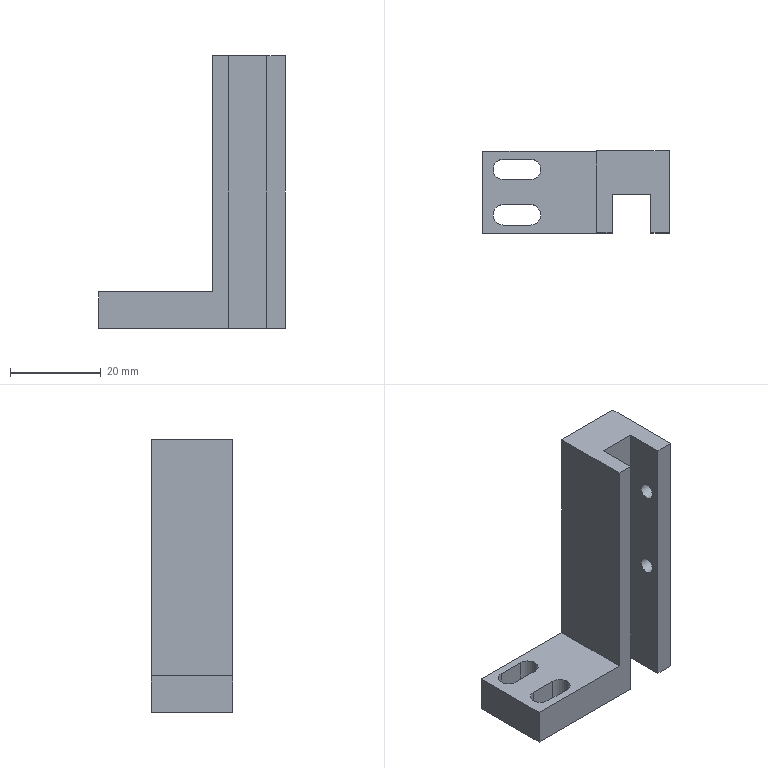Part | NX | features BREP 1 | 1 solid | 22 faces | box 41 x 18 x 60 mm | volume 15782 mm3 | plane 16 | cylinder 6 | commonest cylinder face diameters 4.5 x4 3.5 x2
STEP:
#1=CARTESIAN_POINT('',(-20.5,-9.,-30.));
#2=VERTEX_POINT('',#1);
#3=CARTESIAN_POINT('',(8.,-9.,-30.));
#4=VERTEX_POINT('',#3);
#5=CARTESIAN_POINT('',(-20.5,-9.,-30.));
#6=DIRECTION('',(1.,0.,0.));
#7=VECTOR('',#6,1000.);
#8=LINE('',#5,#7);
#9=EDGE_CURVE('',#2,#4,#8,.T.);
#10=ORIENTED_EDGE('',*,*,#9,.T.);
#11=CARTESIAN_POINT('',(8.,-9.,30.));
#12=VERTEX_POINT('',#11);
#13=CARTESIAN_POINT('',(8.,-9.,-42.021));
#14=DIRECTION('',(0.,0.,1.));
#15=VECTOR('',#14,1000.);
#16=LINE('',#13,#15);
#17=EDGE_CURVE('',#4,#12,#16,.T.);
#18=ORIENTED_EDGE('',*,*,#17,.T.);
#19=CARTESIAN_POINT('',(4.5,-9.,30.));
#20=VERTEX_POINT('',#19);
#21=CARTESIAN_POINT('',(-20.5,-9.,30.));
#22=DIRECTION('',(1.,0.,0.));
#23=VECTOR('',#22,1000.);
#24=LINE('',#21,#23);
#25=EDGE_CURVE('',#20,#12,#24,.T.);
#26=ORIENTED_EDGE('',*,*,#25,.F.);
#27=CARTESIAN_POINT('',(4.5,-9.,-22.));
#28=VERTEX_POINT('',#27);
#29=CARTESIAN_POINT('',(4.5,-9.,30.));
#30=DIRECTION('',(0.,0.,1.));
#31=VECTOR('',#30,1000.);
#32=LINE('',#29,#31);
#33=EDGE_CURVE('',#28,#20,#32,.T.);
#34=ORIENTED_EDGE('',*,*,#33,.F.);
#35=CARTESIAN_POINT('',(-20.5,-9.,-22.));
#36=VERTEX_POINT('',#35);
#37=CARTESIAN_POINT('',(-20.5,-9.,-22.));
#38=DIRECTION('',(1.,0.,0.));
#39=VECTOR('',#38,1000.);
#40=LINE('',#37,#39);
#41=EDGE_CURVE('',#36,#28,#40,.T.);
#42=ORIENTED_EDGE('',*,*,#41,.F.);
#43=CARTESIAN_POINT('',(-20.5,-9.,30.));
#44=DIRECTION('',(0.,0.,-1.));
#45=VECTOR('',#44,1000.);
#46=LINE('',#43,#45);
#47=EDGE_CURVE('',#36,#2,#46,.T.);
#48=ORIENTED_EDGE('',*,*,#47,.T.);
#49=EDGE_LOOP('',(#10,#18,#26,#34,#42,#48));
#50=FACE_BOUND('',#49,.T.);
#51=CARTESIAN_POINT('',(-20.5,-9.,30.));
#52=DIRECTION('',(0.,1.,0.));
#53=DIRECTION('',(0.,0.,-1.));
#54=AXIS2_PLACEMENT_3D('',#51,#52,#53);
#55=PLANE('',#54);
#56=ADVANCED_FACE('',(#50),#55,.F.);
#57=CARTESIAN_POINT('',(20.5,-5.5,-4.45));
#58=VERTEX_POINT('',#57);
#59=CARTESIAN_POINT('',(20.5,-5.5,-2.7));
#60=DIRECTION('',(1.,0.,0.));
#61=DIRECTION('',(0.,0.,-1.));
#62=AXIS2_PLACEMENT_3D('',#59,#60,#61);
#63=CIRCLE('',#62,1.75);
#64=EDGE_CURVE('',#58,#58,#63,.T.);
#65=ORIENTED_EDGE('',*,*,#64,.F.);
#66=EDGE_LOOP('',(#65));
#67=FACE_BOUND('',#66,.T.);
#68=CARTESIAN_POINT('',(20.5,-5.5,15.55));
#69=VERTEX_POINT('',#68);
#70=CARTESIAN_POINT('',(20.5,-5.5,17.3));
#71=DIRECTION('',(1.,0.,0.));
#72=DIRECTION('',(0.,0.,-1.));
#73=AXIS2_PLACEMENT_3D('',#70,#71,#72);
#74=CIRCLE('',#73,1.75);
#75=EDGE_CURVE('',#69,#69,#74,.T.);
#76=ORIENTED_EDGE('',*,*,#75,.F.);
#77=EDGE_LOOP('',(#76));
#78=FACE_BOUND('',#77,.T.);
#79=CARTESIAN_POINT('',(20.5,-9.,-30.));
#80=VERTEX_POINT('',#79);
#81=CARTESIAN_POINT('',(20.5,9.,-30.));
#82=VERTEX_POINT('',#81);
#83=CARTESIAN_POINT('',(20.5,-9.,-30.));
#84=DIRECTION('',(0.,1.,0.));
#85=VECTOR('',#84,1000.);
#86=LINE('',#83,#85);
#87=EDGE_CURVE('',#80,#82,#86,.T.);
#88=ORIENTED_EDGE('',*,*,#87,.T.);
#89=CARTESIAN_POINT('',(20.5,9.,30.));
#90=VERTEX_POINT('',#89);
#91=CARTESIAN_POINT('',(20.5,9.,30.));
#92=DIRECTION('',(0.,0.,-1.));
#93=VECTOR('',#92,1000.);
#94=LINE('',#91,#93);
#95=EDGE_CURVE('',#90,#82,#94,.T.);
#96=ORIENTED_EDGE('',*,*,#95,.F.);
#97=CARTESIAN_POINT('',(20.5,-9.,30.));
#98=VERTEX_POINT('',#97);
#99=CARTESIAN_POINT('',(20.5,-9.,30.));
#100=DIRECTION('',(0.,1.,0.));
#101=VECTOR('',#100,1000.);
#102=LINE('',#99,#101);
#103=EDGE_CURVE('',#98,#90,#102,.T.);
#104=ORIENTED_EDGE('',*,*,#103,.F.);
#105=CARTESIAN_POINT('',(20.5,-9.,30.));
#106=DIRECTION('',(0.,0.,-1.));
#107=VECTOR('',#106,1000.);
#108=LINE('',#105,#107);
#109=EDGE_CURVE('',#98,#80,#108,.T.);
#110=ORIENTED_EDGE('',*,*,#109,.T.);
#111=EDGE_LOOP('',(#88,#96,#104,#110));
#112=FACE_BOUND('',#111,.T.);
#113=CARTESIAN_POINT('',(20.5,-9.,30.));
#114=DIRECTION('',(-1.,0.,0.));
#115=DIRECTION('',(0.,0.,-1.));
#116=AXIS2_PLACEMENT_3D('',#113,#114,#115);
#117=PLANE('',#116);
#118=ADVANCED_FACE('',(#67,#78,#112),#117,.F.);
#119=CARTESIAN_POINT('',(-20.5,9.,-22.));
#120=VERTEX_POINT('',#119);
#121=CARTESIAN_POINT('',(-20.5,9.,-30.));
#122=VERTEX_POINT('',#121);
#123=CARTESIAN_POINT('',(-20.5,9.,30.));
#124=DIRECTION('',(0.,0.,-1.));
#125=VECTOR('',#124,1000.);
#126=LINE('',#123,#125);
#127=EDGE_CURVE('',#120,#122,#126,.T.);
#128=ORIENTED_EDGE('',*,*,#127,.F.);
#129=CARTESIAN_POINT('',(4.5,9.,-22.));
#130=VERTEX_POINT('',#129);
#131=CARTESIAN_POINT('',(-20.5,9.,-22.));
#132=DIRECTION('',(-1.,0.,0.));
#133=VECTOR('',#132,1000.);
#134=LINE('',#131,#133);
#135=EDGE_CURVE('',#130,#120,#134,.T.);
#136=ORIENTED_EDGE('',*,*,#135,.F.);
#137=CARTESIAN_POINT('',(4.5,9.,30.));
#138=VERTEX_POINT('',#137);
#139=CARTESIAN_POINT('',(4.5,9.,30.));
#140=DIRECTION('',(0.,0.,-1.));
#141=VECTOR('',#140,1000.);
#142=LINE('',#139,#141);
#143=EDGE_CURVE('',#138,#130,#142,.T.);
#144=ORIENTED_EDGE('',*,*,#143,.F.);
#145=CARTESIAN_POINT('',(-20.5,9.,30.));
#146=DIRECTION('',(-1.,0.,0.));
#147=VECTOR('',#146,1000.);
#148=LINE('',#145,#147);
#149=EDGE_CURVE('',#90,#138,#148,.T.);
#150=ORIENTED_EDGE('',*,*,#149,.F.);
#151=ORIENTED_EDGE('',*,*,#95,.T.);
#152=CARTESIAN_POINT('',(-20.5,9.,-30.));
#153=DIRECTION('',(-1.,0.,0.));
#154=VECTOR('',#153,1000.);
#155=LINE('',#152,#154);
#156=EDGE_CURVE('',#82,#122,#155,.T.);
#157=ORIENTED_EDGE('',*,*,#156,.T.);
#158=EDGE_LOOP('',(#128,#136,#144,#150,#151,#157));
#159=FACE_BOUND('',#158,.T.);
#160=CARTESIAN_POINT('',(-20.5,9.,30.));
#161=DIRECTION('',(0.,-1.,0.));
#162=DIRECTION('',(0.,0.,1.));
#163=AXIS2_PLACEMENT_3D('',#160,#161,#162);
#164=PLANE('',#163);
#165=ADVANCED_FACE('',(#159),#164,.F.);
#166=ORIENTED_EDGE('',*,*,#47,.F.);
#167=CARTESIAN_POINT('',(-20.5,-66.697,-22.));
#168=DIRECTION('',(0.,1.,0.));
#169=VECTOR('',#168,1000.);
#170=LINE('',#167,#169);
#171=EDGE_CURVE('',#36,#120,#170,.T.);
#172=ORIENTED_EDGE('',*,*,#171,.T.);
#173=ORIENTED_EDGE('',*,*,#127,.T.);
#174=CARTESIAN_POINT('',(-20.5,-9.,-30.));
#175=DIRECTION('',(0.,-1.,0.));
#176=VECTOR('',#175,1000.);
#177=LINE('',#174,#176);
#178=EDGE_CURVE('',#122,#2,#177,.T.);
#179=ORIENTED_EDGE('',*,*,#178,.T.);
#180=EDGE_LOOP('',(#166,#172,#173,#179));
#181=FACE_BOUND('',#180,.T.);
#182=CARTESIAN_POINT('',(-20.5,-9.,30.));
#183=DIRECTION('',(1.,0.,0.));
#184=DIRECTION('',(0.,0.,1.));
#185=AXIS2_PLACEMENT_3D('',#182,#183,#184);
#186=PLANE('',#185);
#187=ADVANCED_FACE('',(#181),#186,.F.);
#188=CARTESIAN_POINT('',(16.5,-9.,30.));
#189=VERTEX_POINT('',#188);
#190=CARTESIAN_POINT('',(-20.5,-9.,30.));
#191=DIRECTION('',(1.,0.,0.));
#192=VECTOR('',#191,1000.);
#193=LINE('',#190,#192);
#194=EDGE_CURVE('',#189,#98,#193,.T.);
#195=ORIENTED_EDGE('',*,*,#194,.F.);
#196=CARTESIAN_POINT('',(16.5,-9.,-30.));
#197=VERTEX_POINT('',#196);
#198=CARTESIAN_POINT('',(16.5,-9.,-42.021));
#199=DIRECTION('',(0.,0.,1.));
#200=VECTOR('',#199,1000.);
#201=LINE('',#198,#200);
#202=EDGE_CURVE('',#197,#189,#201,.T.);
#203=ORIENTED_EDGE('',*,*,#202,.F.);
#204=CARTESIAN_POINT('',(-20.5,-9.,-30.));
#205=DIRECTION('',(1.,0.,0.));
#206=VECTOR('',#205,1000.);
#207=LINE('',#204,#206);
#208=EDGE_CURVE('',#197,#80,#207,.T.);
#209=ORIENTED_EDGE('',*,*,#208,.T.);
#210=ORIENTED_EDGE('',*,*,#109,.F.);
#211=EDGE_LOOP('',(#195,#203,#209,#210));
#212=FACE_BOUND('',#211,.T.);
#213=CARTESIAN_POINT('',(-20.5,-9.,30.));
#214=DIRECTION('',(0.,1.,0.));
#215=DIRECTION('',(0.,0.,-1.));
#216=AXIS2_PLACEMENT_3D('',#213,#214,#215);
#217=PLANE('',#216);
#218=ADVANCED_FACE('',(#212),#217,.F.);
#219=ORIENTED_EDGE('',*,*,#25,.T.);
#220=CARTESIAN_POINT('',(8.,-0.5,30.));
#221=VERTEX_POINT('',#220);
#222=CARTESIAN_POINT('',(8.,-9.,30.));
#223=DIRECTION('',(0.,-1.,0.));
#224=VECTOR('',#223,1000.);
#225=LINE('',#222,#224);
#226=EDGE_CURVE('',#221,#12,#225,.T.);
#227=ORIENTED_EDGE('',*,*,#226,.F.);
#228=CARTESIAN_POINT('',(16.5,-0.5,30.));
#229=VERTEX_POINT('',#228);
#230=CARTESIAN_POINT('',(16.5,-0.5,30.));
#231=DIRECTION('',(-1.,0.,0.));
#232=VECTOR('',#231,1000.);
#233=LINE('',#230,#232);
#234=EDGE_CURVE('',#229,#221,#233,.T.);
#235=ORIENTED_EDGE('',*,*,#234,.F.);
#236=CARTESIAN_POINT('',(16.5,-9.,30.));
#237=DIRECTION('',(0.,1.,0.));
#238=VECTOR('',#237,1000.);
#239=LINE('',#236,#238);
#240=EDGE_CURVE('',#189,#229,#239,.T.);
#241=ORIENTED_EDGE('',*,*,#240,.F.);
#242=ORIENTED_EDGE('',*,*,#194,.T.);
#243=ORIENTED_EDGE('',*,*,#103,.T.);
#244=ORIENTED_EDGE('',*,*,#149,.T.);
#245=CARTESIAN_POINT('',(4.5,-66.697,30.));
#246=DIRECTION('',(0.,1.,0.));
#247=VECTOR('',#246,1000.);
#248=LINE('',#245,#247);
#249=EDGE_CURVE('',#20,#138,#248,.T.);
#250=ORIENTED_EDGE('',*,*,#249,.F.);
#251=EDGE_LOOP('',(#219,#227,#235,#241,#242,#243,#244,#250));
#252=FACE_BOUND('',#251,.T.);
#253=CARTESIAN_POINT('',(0.,0.,30.));
#254=DIRECTION('',(0.,0.,-1.));
#255=DIRECTION('',(1.,0.,0.));
#256=AXIS2_PLACEMENT_3D('',#253,#254,#255);
#257=PLANE('',#256);
#258=ADVANCED_FACE('',(#252),#257,.F.);
#259=CARTESIAN_POINT('',(-16.,-7.25,-30.));
#260=VERTEX_POINT('',#259);
#261=CARTESIAN_POINT('',(-16.,-2.75,-30.));
#262=VERTEX_POINT('',#261);
#263=CARTESIAN_POINT('',(-16.,-5.,-30.));
#264=DIRECTION('',(0.,0.,-1.));
#265=DIRECTION('',(-1.,0.,0.));
#266=AXIS2_PLACEMENT_3D('',#263,#264,#265);
#267=CIRCLE('',#266,2.25);
#268=EDGE_CURVE('',#260,#262,#267,.T.);
#269=ORIENTED_EDGE('',*,*,#268,.F.);
#270=CARTESIAN_POINT('',(-10.,-7.25,-30.));
#271=VERTEX_POINT('',#270);
#272=CARTESIAN_POINT('',(-16.,-7.25,-30.));
#273=DIRECTION('',(-1.,0.,0.));
#274=VECTOR('',#273,1000.);
#275=LINE('',#272,#274);
#276=EDGE_CURVE('',#271,#260,#275,.T.);
#277=ORIENTED_EDGE('',*,*,#276,.F.);
#278=CARTESIAN_POINT('',(-10.,-2.75,-30.));
#279=VERTEX_POINT('',#278);
#280=CARTESIAN_POINT('',(-10.,-5.,-30.));
#281=DIRECTION('',(0.,0.,-1.));
#282=DIRECTION('',(-1.,0.,0.));
#283=AXIS2_PLACEMENT_3D('',#280,#281,#282);
#284=CIRCLE('',#283,2.25);
#285=EDGE_CURVE('',#279,#271,#284,.T.);
#286=ORIENTED_EDGE('',*,*,#285,.F.);
#287=CARTESIAN_POINT('',(-16.,-2.75,-30.));
#288=DIRECTION('',(1.,0.,0.));
#289=VECTOR('',#288,1000.);
#290=LINE('',#287,#289);
#291=EDGE_CURVE('',#262,#279,#290,.T.);
#292=ORIENTED_EDGE('',*,*,#291,.F.);
#293=EDGE_LOOP('',(#269,#277,#286,#292));
#294=FACE_BOUND('',#293,.T.);
#295=CARTESIAN_POINT('',(-16.,2.75,-30.));
#296=VERTEX_POINT('',#295);
#297=CARTESIAN_POINT('',(-16.,7.25,-30.));
#298=VERTEX_POINT('',#297);
#299=CARTESIAN_POINT('',(-16.,5.,-30.));
#300=DIRECTION('',(0.,0.,-1.));
#301=DIRECTION('',(-1.,0.,0.));
#302=AXIS2_PLACEMENT_3D('',#299,#300,#301);
#303=CIRCLE('',#302,2.25);
#304=EDGE_CURVE('',#296,#298,#303,.T.);
#305=ORIENTED_EDGE('',*,*,#304,.F.);
#306=CARTESIAN_POINT('',(-10.,2.75,-30.));
#307=VERTEX_POINT('',#306);
#308=CARTESIAN_POINT('',(-16.,2.75,-30.));
#309=DIRECTION('',(-1.,0.,0.));
#310=VECTOR('',#309,1000.);
#311=LINE('',#308,#310);
#312=EDGE_CURVE('',#307,#296,#311,.T.);
#313=ORIENTED_EDGE('',*,*,#312,.F.);
#314=CARTESIAN_POINT('',(-10.,7.25,-30.));
#315=VERTEX_POINT('',#314);
#316=CARTESIAN_POINT('',(-10.,5.,-30.));
#317=DIRECTION('',(0.,0.,-1.));
#318=DIRECTION('',(-1.,0.,0.));
#319=AXIS2_PLACEMENT_3D('',#316,#317,#318);
#320=CIRCLE('',#319,2.25);
#321=EDGE_CURVE('',#315,#307,#320,.T.);
#322=ORIENTED_EDGE('',*,*,#321,.F.);
#323=CARTESIAN_POINT('',(-16.,7.25,-30.));
#324=DIRECTION('',(1.,0.,0.));
#325=VECTOR('',#324,1000.);
#326=LINE('',#323,#325);
#327=EDGE_CURVE('',#298,#315,#326,.T.);
#328=ORIENTED_EDGE('',*,*,#327,.F.);
#329=EDGE_LOOP('',(#305,#313,#322,#328));
#330=FACE_BOUND('',#329,.T.);
#331=CARTESIAN_POINT('',(8.,-0.5,-30.));
#332=VERTEX_POINT('',#331);
#333=CARTESIAN_POINT('',(8.,-9.,-30.));
#334=DIRECTION('',(0.,-1.,0.));
#335=VECTOR('',#334,1000.);
#336=LINE('',#333,#335);
#337=EDGE_CURVE('',#332,#4,#336,.T.);
#338=ORIENTED_EDGE('',*,*,#337,.T.);
#339=ORIENTED_EDGE('',*,*,#9,.F.);
#340=ORIENTED_EDGE('',*,*,#178,.F.);
#341=ORIENTED_EDGE('',*,*,#156,.F.);
#342=ORIENTED_EDGE('',*,*,#87,.F.);
#343=ORIENTED_EDGE('',*,*,#208,.F.);
#344=CARTESIAN_POINT('',(16.5,-0.5,-30.));
#345=VERTEX_POINT('',#344);
#346=CARTESIAN_POINT('',(16.5,-9.,-30.));
#347=DIRECTION('',(0.,1.,0.));
#348=VECTOR('',#347,1000.);
#349=LINE('',#346,#348);
#350=EDGE_CURVE('',#197,#345,#349,.T.);
#351=ORIENTED_EDGE('',*,*,#350,.T.);
#352=CARTESIAN_POINT('',(16.5,-0.5,-30.));
#353=DIRECTION('',(-1.,0.,0.));
#354=VECTOR('',#353,1000.);
#355=LINE('',#352,#354);
#356=EDGE_CURVE('',#345,#332,#355,.T.);
#357=ORIENTED_EDGE('',*,*,#356,.T.);
#358=EDGE_LOOP('',(#338,#339,#340,#341,#342,#343,#351,#357));
#359=FACE_BOUND('',#358,.T.);
#360=CARTESIAN_POINT('',(0.,0.,-30.));
#361=DIRECTION('',(0.,0.,-1.));
#362=DIRECTION('',(1.,0.,0.));
#363=AXIS2_PLACEMENT_3D('',#360,#361,#362);
#364=PLANE('',#363);
#365=ADVANCED_FACE('',(#294,#330,#359),#364,.T.);
#366=CARTESIAN_POINT('',(-16.,-7.25,-22.));
#367=VERTEX_POINT('',#366);
#368=CARTESIAN_POINT('',(-10.,-7.25,-22.));
#369=VERTEX_POINT('',#368);
#370=CARTESIAN_POINT('',(-16.,-7.25,-22.));
#371=DIRECTION('',(1.,0.,0.));
#372=VECTOR('',#371,1000.);
#373=LINE('',#370,#372);
#374=EDGE_CURVE('',#367,#369,#373,.T.);
#375=ORIENTED_EDGE('',*,*,#374,.F.);
#376=CARTESIAN_POINT('',(-16.,-2.75,-22.));
#377=VERTEX_POINT('',#376);
#378=CARTESIAN_POINT('',(-16.,-5.,-22.));
#379=DIRECTION('',(0.,0.,1.));
#380=DIRECTION('',(-1.,0.,0.));
#381=AXIS2_PLACEMENT_3D('',#378,#379,#380);
#382=CIRCLE('',#381,2.25);
#383=EDGE_CURVE('',#377,#367,#382,.T.);
#384=ORIENTED_EDGE('',*,*,#383,.F.);
#385=CARTESIAN_POINT('',(-10.,-2.75,-22.));
#386=VERTEX_POINT('',#385);
#387=CARTESIAN_POINT('',(-16.,-2.75,-22.));
#388=DIRECTION('',(-1.,0.,0.));
#389=VECTOR('',#388,1000.);
#390=LINE('',#387,#389);
#391=EDGE_CURVE('',#386,#377,#390,.T.);
#392=ORIENTED_EDGE('',*,*,#391,.F.);
#393=CARTESIAN_POINT('',(-10.,-5.,-22.));
#394=DIRECTION('',(0.,0.,1.));
#395=DIRECTION('',(-1.,0.,0.));
#396=AXIS2_PLACEMENT_3D('',#393,#394,#395);
#397=CIRCLE('',#396,2.25);
#398=EDGE_CURVE('',#369,#386,#397,.T.);
#399=ORIENTED_EDGE('',*,*,#398,.F.);
#400=EDGE_LOOP('',(#375,#384,#392,#399));
#401=FACE_BOUND('',#400,.T.);
#402=CARTESIAN_POINT('',(-16.,2.75,-22.));
#403=VERTEX_POINT('',#402);
#404=CARTESIAN_POINT('',(-10.,2.75,-22.));
#405=VERTEX_POINT('',#404);
#406=CARTESIAN_POINT('',(-16.,2.75,-22.));
#407=DIRECTION('',(1.,0.,0.));
#408=VECTOR('',#407,1000.);
#409=LINE('',#406,#408);
#410=EDGE_CURVE('',#403,#405,#409,.T.);
#411=ORIENTED_EDGE('',*,*,#410,.F.);
#412=CARTESIAN_POINT('',(-16.,7.25,-22.));
#413=VERTEX_POINT('',#412);
#414=CARTESIAN_POINT('',(-16.,5.,-22.));
#415=DIRECTION('',(0.,0.,1.));
#416=DIRECTION('',(-1.,0.,0.));
#417=AXIS2_PLACEMENT_3D('',#414,#415,#416);
#418=CIRCLE('',#417,2.25);
#419=EDGE_CURVE('',#413,#403,#418,.T.);
#420=ORIENTED_EDGE('',*,*,#419,.F.);
#421=CARTESIAN_POINT('',(-10.,7.25,-22.));
#422=VERTEX_POINT('',#421);
#423=CARTESIAN_POINT('',(-16.,7.25,-22.));
#424=DIRECTION('',(-1.,0.,0.));
#425=VECTOR('',#424,1000.);
#426=LINE('',#423,#425);
#427=EDGE_CURVE('',#422,#413,#426,.T.);
#428=ORIENTED_EDGE('',*,*,#427,.F.);
#429=CARTESIAN_POINT('',(-10.,5.,-22.));
#430=DIRECTION('',(0.,0.,1.));
#431=DIRECTION('',(-1.,0.,0.));
#432=AXIS2_PLACEMENT_3D('',#429,#430,#431);
#433=CIRCLE('',#432,2.25);
#434=EDGE_CURVE('',#405,#422,#433,.T.);
#435=ORIENTED_EDGE('',*,*,#434,.F.);
#436=EDGE_LOOP('',(#411,#420,#428,#435));
#437=FACE_BOUND('',#436,.T.);
#438=ORIENTED_EDGE('',*,*,#41,.T.);
#439=CARTESIAN_POINT('',(4.5,-66.697,-22.));
#440=DIRECTION('',(0.,1.,0.));
#441=VECTOR('',#440,1000.);
#442=LINE('',#439,#441);
#443=EDGE_CURVE('',#28,#130,#442,.T.);
#444=ORIENTED_EDGE('',*,*,#443,.T.);
#445=ORIENTED_EDGE('',*,*,#135,.T.);
#446=ORIENTED_EDGE('',*,*,#171,.F.);
#447=EDGE_LOOP('',(#438,#444,#445,#446));
#448=FACE_BOUND('',#447,.T.);
#449=CARTESIAN_POINT('',(-20.5,-66.697,-22.));
#450=DIRECTION('',(0.,0.,-1.));
#451=DIRECTION('',(1.,0.,0.));
#452=AXIS2_PLACEMENT_3D('',#449,#450,#451);
#453=PLANE('',#452);
#454=ADVANCED_FACE('',(#401,#437,#448),#453,.F.);
#455=ORIENTED_EDGE('',*,*,#33,.T.);
#456=ORIENTED_EDGE('',*,*,#249,.T.);
#457=ORIENTED_EDGE('',*,*,#143,.T.);
#458=ORIENTED_EDGE('',*,*,#443,.F.);
#459=EDGE_LOOP('',(#455,#456,#457,#458));
#460=FACE_BOUND('',#459,.T.);
#461=CARTESIAN_POINT('',(4.5,-66.697,30.));
#462=DIRECTION('',(1.,0.,0.));
#463=DIRECTION('',(0.,0.,1.));
#464=AXIS2_PLACEMENT_3D('',#461,#462,#463);
#465=PLANE('',#464);
#466=ADVANCED_FACE('',(#460),#465,.F.);
#467=CARTESIAN_POINT('',(16.5,-0.5,-42.021));
#468=DIRECTION('',(0.,0.,1.));
#469=VECTOR('',#468,1000.);
#470=LINE('',#467,#469);
#471=EDGE_CURVE('',#345,#229,#470,.T.);
#472=ORIENTED_EDGE('',*,*,#471,.T.);
#473=ORIENTED_EDGE('',*,*,#234,.T.);
#474=CARTESIAN_POINT('',(8.,-0.5,-42.021));
#475=DIRECTION('',(0.,0.,1.));
#476=VECTOR('',#475,1000.);
#477=LINE('',#474,#476);
#478=EDGE_CURVE('',#332,#221,#477,.T.);
#479=ORIENTED_EDGE('',*,*,#478,.F.);
#480=ORIENTED_EDGE('',*,*,#356,.F.);
#481=EDGE_LOOP('',(#472,#473,#479,#480));
#482=FACE_BOUND('',#481,.T.);
#483=CARTESIAN_POINT('',(16.5,-0.5,-42.021));
#484=DIRECTION('',(0.,1.,0.));
#485=DIRECTION('',(1.,0.,0.));
#486=AXIS2_PLACEMENT_3D('',#483,#484,#485);
#487=PLANE('',#486);
#488=ADVANCED_FACE('',(#482),#487,.F.);
#489=ORIENTED_EDGE('',*,*,#478,.T.);
#490=ORIENTED_EDGE('',*,*,#226,.T.);
#491=ORIENTED_EDGE('',*,*,#17,.F.);
#492=ORIENTED_EDGE('',*,*,#337,.F.);
#493=EDGE_LOOP('',(#489,#490,#491,#492));
#494=FACE_BOUND('',#493,.T.);
#495=CARTESIAN_POINT('',(8.,-9.,-42.021));
#496=DIRECTION('',(-1.,0.,0.));
#497=DIRECTION('',(0.,0.,-1.));
#498=AXIS2_PLACEMENT_3D('',#495,#496,#497);
#499=PLANE('',#498);
#500=ADVANCED_FACE('',(#494),#499,.F.);
#501=CARTESIAN_POINT('',(16.5,-5.5,-4.45));
#502=VERTEX_POINT('',#501);
#503=CARTESIAN_POINT('',(16.5,-5.5,-2.7));
#504=DIRECTION('',(1.,0.,0.));
#505=DIRECTION('',(0.,0.,-1.));
#506=AXIS2_PLACEMENT_3D('',#503,#504,#505);
#507=CIRCLE('',#506,1.75);
#508=EDGE_CURVE('',#502,#502,#507,.T.);
#509=ORIENTED_EDGE('',*,*,#508,.T.);
#510=EDGE_LOOP('',(#509));
#511=FACE_BOUND('',#510,.T.);
#512=CARTESIAN_POINT('',(16.5,-5.5,15.55));
#513=VERTEX_POINT('',#512);
#514=CARTESIAN_POINT('',(16.5,-5.5,17.3));
#515=DIRECTION('',(1.,0.,0.));
#516=DIRECTION('',(0.,0.,-1.));
#517=AXIS2_PLACEMENT_3D('',#514,#515,#516);
#518=CIRCLE('',#517,1.75);
#519=EDGE_CURVE('',#513,#513,#518,.T.);
#520=ORIENTED_EDGE('',*,*,#519,.T.);
#521=EDGE_LOOP('',(#520));
#522=FACE_BOUND('',#521,.T.);
#523=ORIENTED_EDGE('',*,*,#202,.T.);
#524=ORIENTED_EDGE('',*,*,#240,.T.);
#525=ORIENTED_EDGE('',*,*,#471,.F.);
#526=ORIENTED_EDGE('',*,*,#350,.F.);
#527=EDGE_LOOP('',(#523,#524,#525,#526));
#528=FACE_BOUND('',#527,.T.);
#529=CARTESIAN_POINT('',(16.5,-9.,-42.021));
#530=DIRECTION('',(1.,0.,0.));
#531=DIRECTION('',(0.,0.,1.));
#532=AXIS2_PLACEMENT_3D('',#529,#530,#531);
#533=PLANE('',#532);
#534=ADVANCED_FACE('',(#511,#522,#528),#533,.F.);
#535=ORIENTED_EDGE('',*,*,#419,.T.);
#536=CARTESIAN_POINT('',(-16.,2.75,-10.576));
#537=DIRECTION('',(0.,0.,-1.));
#538=VECTOR('',#537,1000.);
#539=LINE('',#536,#538);
#540=EDGE_CURVE('',#403,#296,#539,.T.);
#541=ORIENTED_EDGE('',*,*,#540,.T.);
#542=ORIENTED_EDGE('',*,*,#304,.T.);
#543=CARTESIAN_POINT('',(-16.,7.25,-10.576));
#544=DIRECTION('',(0.,0.,-1.));
#545=VECTOR('',#544,1000.);
#546=LINE('',#543,#545);
#547=EDGE_CURVE('',#413,#298,#546,.T.);
#548=ORIENTED_EDGE('',*,*,#547,.F.);
#549=EDGE_LOOP('',(#535,#541,#542,#548));
#550=FACE_BOUND('',#549,.T.);
#551=CARTESIAN_POINT('',(-16.,5.,-10.576));
#552=DIRECTION('',(0.,0.,-1.));
#553=DIRECTION('',(1.,0.,0.));
#554=AXIS2_PLACEMENT_3D('',#551,#552,#553);
#555=CYLINDRICAL_SURFACE('',#554,2.25);
#556=ADVANCED_FACE('',(#550),#555,.F.);
#557=ORIENTED_EDGE('',*,*,#410,.T.);
#558=CARTESIAN_POINT('',(-10.,2.75,-10.576));
#559=DIRECTION('',(0.,0.,-1.));
#560=VECTOR('',#559,1000.);
#561=LINE('',#558,#560);
#562=EDGE_CURVE('',#405,#307,#561,.T.);
#563=ORIENTED_EDGE('',*,*,#562,.T.);
#564=ORIENTED_EDGE('',*,*,#312,.T.);
#565=ORIENTED_EDGE('',*,*,#540,.F.);
#566=EDGE_LOOP('',(#557,#563,#564,#565));
#567=FACE_BOUND('',#566,.T.);
#568=CARTESIAN_POINT('',(-16.,2.75,-10.576));
#569=DIRECTION('',(0.,-1.,0.));
#570=DIRECTION('',(-1.,0.,0.));
#571=AXIS2_PLACEMENT_3D('',#568,#569,#570);
#572=PLANE('',#571);
#573=ADVANCED_FACE('',(#567),#572,.F.);
#574=ORIENTED_EDGE('',*,*,#434,.T.);
#575=CARTESIAN_POINT('',(-10.,7.25,-10.576));
#576=DIRECTION('',(0.,0.,-1.));
#577=VECTOR('',#576,1000.);
#578=LINE('',#575,#577);
#579=EDGE_CURVE('',#422,#315,#578,.T.);
#580=ORIENTED_EDGE('',*,*,#579,.T.);
#581=ORIENTED_EDGE('',*,*,#321,.T.);
#582=ORIENTED_EDGE('',*,*,#562,.F.);
#583=EDGE_LOOP('',(#574,#580,#581,#582));
#584=FACE_BOUND('',#583,.T.);
#585=CARTESIAN_POINT('',(-10.,5.,-10.576));
#586=DIRECTION('',(0.,0.,-1.));
#587=DIRECTION('',(1.,0.,0.));
#588=AXIS2_PLACEMENT_3D('',#585,#586,#587);
#589=CYLINDRICAL_SURFACE('',#588,2.25);
#590=ADVANCED_FACE('',(#584),#589,.F.);
#591=ORIENTED_EDGE('',*,*,#427,.T.);
#592=ORIENTED_EDGE('',*,*,#547,.T.);
#593=ORIENTED_EDGE('',*,*,#327,.T.);
#594=ORIENTED_EDGE('',*,*,#579,.F.);
#595=EDGE_LOOP('',(#591,#592,#593,#594));
#596=FACE_BOUND('',#595,.T.);
#597=CARTESIAN_POINT('',(-16.,7.25,-10.576));
#598=DIRECTION('',(0.,1.,0.));
#599=DIRECTION('',(1.,0.,0.));
#600=AXIS2_PLACEMENT_3D('',#597,#598,#599);
#601=PLANE('',#600);
#602=ADVANCED_FACE('',(#596),#601,.F.);
#603=ORIENTED_EDGE('',*,*,#383,.T.);
#604=CARTESIAN_POINT('',(-16.,-7.25,-10.576));
#605=DIRECTION('',(0.,0.,-1.));
#606=VECTOR('',#605,1000.);
#607=LINE('',#604,#606);
#608=EDGE_CURVE('',#367,#260,#607,.T.);
#609=ORIENTED_EDGE('',*,*,#608,.T.);
#610=ORIENTED_EDGE('',*,*,#268,.T.);
#611=CARTESIAN_POINT('',(-16.,-2.75,-10.576));
#612=DIRECTION('',(0.,0.,-1.));
#613=VECTOR('',#612,1000.);
#614=LINE('',#611,#613);
#615=EDGE_CURVE('',#377,#262,#614,.T.);
#616=ORIENTED_EDGE('',*,*,#615,.F.);
#617=EDGE_LOOP('',(#603,#609,#610,#616));
#618=FACE_BOUND('',#617,.T.);
#619=CARTESIAN_POINT('',(-16.,-5.,-10.576));
#620=DIRECTION('',(0.,0.,-1.));
#621=DIRECTION('',(1.,0.,0.));
#622=AXIS2_PLACEMENT_3D('',#619,#620,#621);
#623=CYLINDRICAL_SURFACE('',#622,2.25);
#624=ADVANCED_FACE('',(#618),#623,.F.);
#625=ORIENTED_EDGE('',*,*,#374,.T.);
#626=CARTESIAN_POINT('',(-10.,-7.25,-10.576));
#627=DIRECTION('',(0.,0.,-1.));
#628=VECTOR('',#627,1000.);
#629=LINE('',#626,#628);
#630=EDGE_CURVE('',#369,#271,#629,.T.);
#631=ORIENTED_EDGE('',*,*,#630,.T.);
#632=ORIENTED_EDGE('',*,*,#276,.T.);
#633=ORIENTED_EDGE('',*,*,#608,.F.);
#634=EDGE_LOOP('',(#625,#631,#632,#633));
#635=FACE_BOUND('',#634,.T.);
#636=CARTESIAN_POINT('',(-16.,-7.25,-10.576));
#637=DIRECTION('',(0.,-1.,0.));
#638=DIRECTION('',(-1.,0.,0.));
#639=AXIS2_PLACEMENT_3D('',#636,#637,#638);
#640=PLANE('',#639);
#641=ADVANCED_FACE('',(#635),#640,.F.);
#642=ORIENTED_EDGE('',*,*,#398,.T.);
#643=CARTESIAN_POINT('',(-10.,-2.75,-10.576));
#644=DIRECTION('',(0.,0.,-1.));
#645=VECTOR('',#644,1000.);
#646=LINE('',#643,#645);
#647=EDGE_CURVE('',#386,#279,#646,.T.);
#648=ORIENTED_EDGE('',*,*,#647,.T.);
#649=ORIENTED_EDGE('',*,*,#285,.T.);
#650=ORIENTED_EDGE('',*,*,#630,.F.);
#651=EDGE_LOOP('',(#642,#648,#649,#650));
#652=FACE_BOUND('',#651,.T.);
#653=CARTESIAN_POINT('',(-10.,-5.,-10.576));
#654=DIRECTION('',(0.,0.,-1.));
#655=DIRECTION('',(1.,0.,0.));
#656=AXIS2_PLACEMENT_3D('',#653,#654,#655);
#657=CYLINDRICAL_SURFACE('',#656,2.25);
#658=ADVANCED_FACE('',(#652),#657,.F.);
#659=ORIENTED_EDGE('',*,*,#391,.T.);
#660=ORIENTED_EDGE('',*,*,#615,.T.);
#661=ORIENTED_EDGE('',*,*,#291,.T.);
#662=ORIENTED_EDGE('',*,*,#647,.F.);
#663=EDGE_LOOP('',(#659,#660,#661,#662));
#664=FACE_BOUND('',#663,.T.);
#665=CARTESIAN_POINT('',(-16.,-2.75,-10.576));
#666=DIRECTION('',(0.,1.,0.));
#667=DIRECTION('',(1.,0.,0.));
#668=AXIS2_PLACEMENT_3D('',#665,#666,#667);
#669=PLANE('',#668);
#670=ADVANCED_FACE('',(#664),#669,.F.);
#671=ORIENTED_EDGE('',*,*,#75,.T.);
#672=EDGE_LOOP('',(#671));
#673=FACE_BOUND('',#672,.T.);
#674=ORIENTED_EDGE('',*,*,#519,.F.);
#675=EDGE_LOOP('',(#674));
#676=FACE_BOUND('',#675,.T.);
#677=CARTESIAN_POINT('',(20.5,-5.5,17.3));
#678=DIRECTION('',(1.,0.,0.));
#679=DIRECTION('',(0.,0.,1.));
#680=AXIS2_PLACEMENT_3D('',#677,#678,#679);
#681=CYLINDRICAL_SURFACE('',#680,1.75);
#682=ADVANCED_FACE('',(#673,#676),#681,.F.);
#683=ORIENTED_EDGE('',*,*,#64,.T.);
#684=EDGE_LOOP('',(#683));
#685=FACE_BOUND('',#684,.T.);
#686=ORIENTED_EDGE('',*,*,#508,.F.);
#687=EDGE_LOOP('',(#686));
#688=FACE_BOUND('',#687,.T.);
#689=CARTESIAN_POINT('',(20.5,-5.5,-2.7));
#690=DIRECTION('',(1.,0.,0.));
#691=DIRECTION('',(0.,0.,1.));
#692=AXIS2_PLACEMENT_3D('',#689,#690,#691);
#693=CYLINDRICAL_SURFACE('',#692,1.75);
#694=ADVANCED_FACE('',(#685,#688),#693,.F.);
#695=CLOSED_SHELL('',(#56,#118,#165,#187,#218,#258,#365,#454,#466,#488,#500,#534,#556,#573,#590,#602,#624,#641,#658,#670,#682,#694));
#696=MANIFOLD_SOLID_BREP('',#695);
#697=(LENGTH_UNIT()NAMED_UNIT(*)SI_UNIT(.MILLI.,.METRE.));
#698=UNCERTAINTY_MEASURE_WITH_UNIT(LENGTH_MEASURE(0.00001),#697,'','');
#699=(NAMED_UNIT(*)PLANE_ANGLE_UNIT()SI_UNIT($,.RADIAN.));
#700=(NAMED_UNIT(*)SI_UNIT($,.STERADIAN.)SOLID_ANGLE_UNIT());
#701=(GEOMETRIC_REPRESENTATION_CONTEXT(3)GLOBAL_UNCERTAINTY_ASSIGNED_CONTEXT((#698))GLOBAL_UNIT_ASSIGNED_CONTEXT((#697,#699,#700))REPRESENTATION_CONTEXT('',''));
#702=ADVANCED_BREP_SHAPE_REPRESENTATION('',(#696),#701);